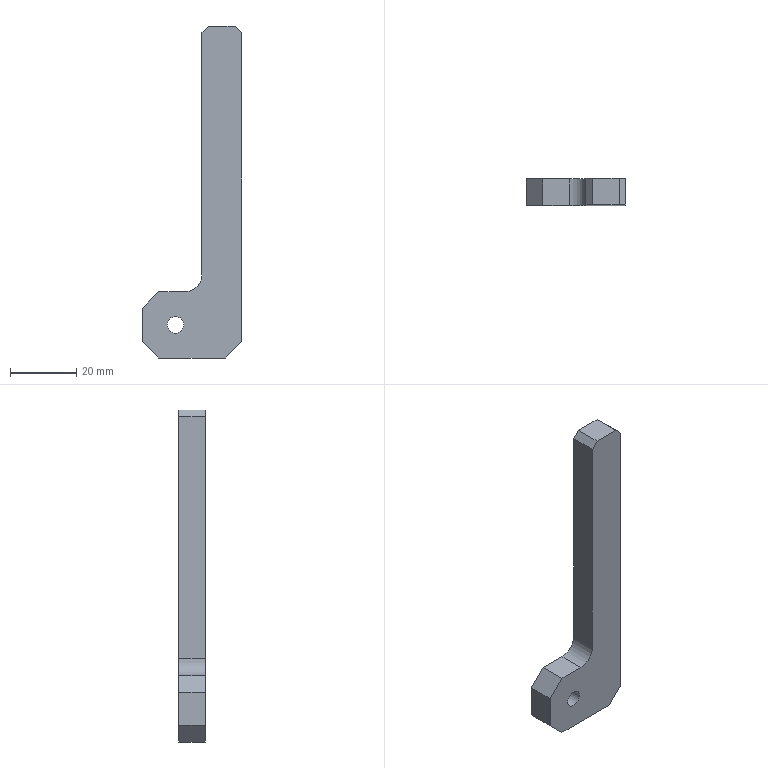Part | NX | features 5003_209_Plate 2 | 1 solid | 15 faces | box 30 x 8 x 100 mm | volume 12034 mm3 | plane 13 | cylinder 2 | commonest cylinder face diameters 5 x1 10 x1
STEP:
#1=CARTESIAN_POINT('',(-208.775,-608.606,-95.5));
#2=VERTEX_POINT('',#1);
#3=CARTESIAN_POINT('',(-208.775,-608.606,-22.5));
#4=VERTEX_POINT('',#3);
#5=CARTESIAN_POINT('',(-208.775,-608.606,-95.5));
#6=DIRECTION('',(0.,0.,1.));
#7=VECTOR('',#6,1000.);
#8=LINE('',#5,#7);
#9=EDGE_CURVE('',#2,#4,#8,.T.);
#10=ORIENTED_EDGE('',*,*,#9,.T.);
#11=CARTESIAN_POINT('',(-206.775,-608.606,-20.5));
#12=VERTEX_POINT('',#11);
#13=CARTESIAN_POINT('',(-247.775,-608.606,-61.5));
#14=DIRECTION('',(-0.7071,0.,-0.7071));
#15=VECTOR('',#14,1000.);
#16=LINE('',#13,#15);
#17=EDGE_CURVE('',#4,#12,#16,.F.);
#18=ORIENTED_EDGE('',*,*,#17,.T.);
#19=CARTESIAN_POINT('',(-198.775,-608.606,-20.5));
#20=VERTEX_POINT('',#19);
#21=CARTESIAN_POINT('',(-196.775,-608.606,-20.5));
#22=DIRECTION('',(1.,0.,0.));
#23=VECTOR('',#22,1000.);
#24=LINE('',#21,#23);
#25=EDGE_CURVE('',#12,#20,#24,.T.);
#26=ORIENTED_EDGE('',*,*,#25,.T.);
#27=CARTESIAN_POINT('',(-196.775,-608.606,-22.5));
#28=VERTEX_POINT('',#27);
#29=CARTESIAN_POINT('',(-168.775,-608.606,-50.5));
#30=DIRECTION('',(-0.7071,0.,0.7071));
#31=VECTOR('',#30,1000.);
#32=LINE('',#29,#31);
#33=EDGE_CURVE('',#20,#28,#32,.F.);
#34=ORIENTED_EDGE('',*,*,#33,.T.);
#35=CARTESIAN_POINT('',(-196.775,-608.606,-115.5));
#36=VERTEX_POINT('',#35);
#37=CARTESIAN_POINT('',(-196.775,-608.606,-115.5));
#38=DIRECTION('',(0.,0.,-1.));
#39=VECTOR('',#38,1000.);
#40=LINE('',#37,#39);
#41=EDGE_CURVE('',#28,#36,#40,.T.);
#42=ORIENTED_EDGE('',*,*,#41,.T.);
#43=CARTESIAN_POINT('',(-201.775,-608.606,-120.5));
#44=VERTEX_POINT('',#43);
#45=CARTESIAN_POINT('',(-201.775,-608.606,-120.5));
#46=DIRECTION('',(-0.7071,0.,-0.7071));
#47=VECTOR('',#46,1000.);
#48=LINE('',#45,#47);
#49=EDGE_CURVE('',#36,#44,#48,.T.);
#50=ORIENTED_EDGE('',*,*,#49,.T.);
#51=CARTESIAN_POINT('',(-221.775,-608.606,-120.5));
#52=VERTEX_POINT('',#51);
#53=CARTESIAN_POINT('',(-201.775,-608.606,-120.5));
#54=DIRECTION('',(-1.,0.,0.));
#55=VECTOR('',#54,1000.);
#56=LINE('',#53,#55);
#57=EDGE_CURVE('',#44,#52,#56,.T.);
#58=ORIENTED_EDGE('',*,*,#57,.T.);
#59=CARTESIAN_POINT('',(-226.775,-608.606,-115.5));
#60=VERTEX_POINT('',#59);
#61=CARTESIAN_POINT('',(-226.775,-608.606,-115.5));
#62=DIRECTION('',(-0.7071,0.,0.7071));
#63=VECTOR('',#62,1000.);
#64=LINE('',#61,#63);
#65=EDGE_CURVE('',#52,#60,#64,.T.);
#66=ORIENTED_EDGE('',*,*,#65,.T.);
#67=CARTESIAN_POINT('',(-226.775,-608.606,-105.5));
#68=VERTEX_POINT('',#67);
#69=CARTESIAN_POINT('',(-226.775,-608.606,-105.5));
#70=DIRECTION('',(0.,0.,1.));
#71=VECTOR('',#70,1000.);
#72=LINE('',#69,#71);
#73=EDGE_CURVE('',#60,#68,#72,.T.);
#74=ORIENTED_EDGE('',*,*,#73,.T.);
#75=CARTESIAN_POINT('',(-221.775,-608.606,-100.5));
#76=VERTEX_POINT('',#75);
#77=CARTESIAN_POINT('',(-221.775,-608.606,-100.5));
#78=DIRECTION('',(0.7071,0.,0.7071));
#79=VECTOR('',#78,1000.);
#80=LINE('',#77,#79);
#81=EDGE_CURVE('',#68,#76,#80,.T.);
#82=ORIENTED_EDGE('',*,*,#81,.T.);
#83=CARTESIAN_POINT('',(-213.775,-608.606,-100.5));
#84=VERTEX_POINT('',#83);
#85=CARTESIAN_POINT('',(-213.775,-608.606,-100.5));
#86=DIRECTION('',(1.,0.,0.));
#87=VECTOR('',#86,1000.);
#88=LINE('',#85,#87);
#89=EDGE_CURVE('',#76,#84,#88,.T.);
#90=ORIENTED_EDGE('',*,*,#89,.T.);
#91=CARTESIAN_POINT('',(-213.775,-608.606,-95.5));
#92=DIRECTION('',(0.,-1.,0.));
#93=DIRECTION('',(-1.,0.,0.));
#94=AXIS2_PLACEMENT_3D('',#91,#92,#93);
#95=CIRCLE('',#94,5.);
#96=EDGE_CURVE('',#84,#2,#95,.T.);
#97=ORIENTED_EDGE('',*,*,#96,.T.);
#98=EDGE_LOOP('',(#10,#18,#26,#34,#42,#50,#58,#66,#74,#82,#90,#97));
#99=FACE_BOUND('',#98,.T.);
#100=CARTESIAN_POINT('',(-219.275,-608.606,-110.5));
#101=VERTEX_POINT('',#100);
#102=CARTESIAN_POINT('',(-216.775,-608.606,-110.5));
#103=DIRECTION('',(0.,1.,0.));
#104=DIRECTION('',(-1.,0.,0.));
#105=AXIS2_PLACEMENT_3D('',#102,#103,#104);
#106=CIRCLE('',#105,2.5);
#107=EDGE_CURVE('',#101,#101,#106,.T.);
#108=ORIENTED_EDGE('',*,*,#107,.F.);
#109=EDGE_LOOP('',(#108));
#110=FACE_BOUND('',#109,.T.);
#111=CARTESIAN_POINT('',(-213.775,-608.606,-95.5));
#112=DIRECTION('',(0.,1.,0.));
#113=DIRECTION('',(-1.,0.,0.));
#114=AXIS2_PLACEMENT_3D('',#111,#112,#113);
#115=PLANE('',#114);
#116=ADVANCED_FACE('',(#99,#110),#115,.T.);
#117=CARTESIAN_POINT('',(-206.775,-616.606,-20.5));
#118=VERTEX_POINT('',#117);
#119=CARTESIAN_POINT('',(-198.775,-616.606,-20.5));
#120=VERTEX_POINT('',#119);
#121=CARTESIAN_POINT('',(-196.775,-616.606,-20.5));
#122=DIRECTION('',(1.,0.,0.));
#123=VECTOR('',#122,1000.);
#124=LINE('',#121,#123);
#125=EDGE_CURVE('',#118,#120,#124,.T.);
#126=ORIENTED_EDGE('',*,*,#125,.F.);
#127=CARTESIAN_POINT('',(-208.775,-616.606,-22.5));
#128=VERTEX_POINT('',#127);
#129=CARTESIAN_POINT('',(-206.775,-616.606,-20.5));
#130=DIRECTION('',(0.7071,0.,0.7071));
#131=VECTOR('',#130,1000.);
#132=LINE('',#129,#131);
#133=EDGE_CURVE('',#118,#128,#132,.F.);
#134=ORIENTED_EDGE('',*,*,#133,.T.);
#135=CARTESIAN_POINT('',(-208.775,-616.606,-95.5));
#136=VERTEX_POINT('',#135);
#137=CARTESIAN_POINT('',(-208.775,-616.606,-95.5));
#138=DIRECTION('',(0.,0.,1.));
#139=VECTOR('',#138,1000.);
#140=LINE('',#137,#139);
#141=EDGE_CURVE('',#136,#128,#140,.T.);
#142=ORIENTED_EDGE('',*,*,#141,.F.);
#143=CARTESIAN_POINT('',(-213.775,-616.606,-100.5));
#144=VERTEX_POINT('',#143);
#145=CARTESIAN_POINT('',(-213.775,-616.606,-95.5));
#146=DIRECTION('',(0.,-1.,0.));
#147=DIRECTION('',(-1.,0.,0.));
#148=AXIS2_PLACEMENT_3D('',#145,#146,#147);
#149=CIRCLE('',#148,5.);
#150=EDGE_CURVE('',#144,#136,#149,.T.);
#151=ORIENTED_EDGE('',*,*,#150,.F.);
#152=CARTESIAN_POINT('',(-221.775,-616.606,-100.5));
#153=VERTEX_POINT('',#152);
#154=CARTESIAN_POINT('',(-213.775,-616.606,-100.5));
#155=DIRECTION('',(1.,0.,0.));
#156=VECTOR('',#155,1000.);
#157=LINE('',#154,#156);
#158=EDGE_CURVE('',#153,#144,#157,.T.);
#159=ORIENTED_EDGE('',*,*,#158,.F.);
#160=CARTESIAN_POINT('',(-226.775,-616.606,-105.5));
#161=VERTEX_POINT('',#160);
#162=CARTESIAN_POINT('',(-221.775,-616.606,-100.5));
#163=DIRECTION('',(0.7071,0.,0.7071));
#164=VECTOR('',#163,1000.);
#165=LINE('',#162,#164);
#166=EDGE_CURVE('',#161,#153,#165,.T.);
#167=ORIENTED_EDGE('',*,*,#166,.F.);
#168=CARTESIAN_POINT('',(-226.775,-616.606,-115.5));
#169=VERTEX_POINT('',#168);
#170=CARTESIAN_POINT('',(-226.775,-616.606,-105.5));
#171=DIRECTION('',(0.,0.,1.));
#172=VECTOR('',#171,1000.);
#173=LINE('',#170,#172);
#174=EDGE_CURVE('',#169,#161,#173,.T.);
#175=ORIENTED_EDGE('',*,*,#174,.F.);
#176=CARTESIAN_POINT('',(-221.775,-616.606,-120.5));
#177=VERTEX_POINT('',#176);
#178=CARTESIAN_POINT('',(-226.775,-616.606,-115.5));
#179=DIRECTION('',(-0.7071,0.,0.7071));
#180=VECTOR('',#179,1000.);
#181=LINE('',#178,#180);
#182=EDGE_CURVE('',#177,#169,#181,.T.);
#183=ORIENTED_EDGE('',*,*,#182,.F.);
#184=CARTESIAN_POINT('',(-201.775,-616.606,-120.5));
#185=VERTEX_POINT('',#184);
#186=CARTESIAN_POINT('',(-201.775,-616.606,-120.5));
#187=DIRECTION('',(-1.,0.,0.));
#188=VECTOR('',#187,1000.);
#189=LINE('',#186,#188);
#190=EDGE_CURVE('',#185,#177,#189,.T.);
#191=ORIENTED_EDGE('',*,*,#190,.F.);
#192=CARTESIAN_POINT('',(-196.775,-616.606,-115.5));
#193=VERTEX_POINT('',#192);
#194=CARTESIAN_POINT('',(-201.775,-616.606,-120.5));
#195=DIRECTION('',(-0.7071,0.,-0.7071));
#196=VECTOR('',#195,1000.);
#197=LINE('',#194,#196);
#198=EDGE_CURVE('',#193,#185,#197,.T.);
#199=ORIENTED_EDGE('',*,*,#198,.F.);
#200=CARTESIAN_POINT('',(-196.775,-616.606,-22.5));
#201=VERTEX_POINT('',#200);
#202=CARTESIAN_POINT('',(-196.775,-616.606,-115.5));
#203=DIRECTION('',(0.,0.,-1.));
#204=VECTOR('',#203,1000.);
#205=LINE('',#202,#204);
#206=EDGE_CURVE('',#201,#193,#205,.T.);
#207=ORIENTED_EDGE('',*,*,#206,.F.);
#208=CARTESIAN_POINT('',(-196.775,-616.606,-22.5));
#209=DIRECTION('',(0.7071,0.,-0.7071));
#210=VECTOR('',#209,1000.);
#211=LINE('',#208,#210);
#212=EDGE_CURVE('',#201,#120,#211,.F.);
#213=ORIENTED_EDGE('',*,*,#212,.T.);
#214=EDGE_LOOP('',(#126,#134,#142,#151,#159,#167,#175,#183,#191,#199,#207,#213));
#215=FACE_BOUND('',#214,.T.);
#216=CARTESIAN_POINT('',(-219.275,-616.606,-110.5));
#217=VERTEX_POINT('',#216);
#218=CARTESIAN_POINT('',(-216.775,-616.606,-110.5));
#219=DIRECTION('',(0.,1.,0.));
#220=DIRECTION('',(-1.,0.,0.));
#221=AXIS2_PLACEMENT_3D('',#218,#219,#220);
#222=CIRCLE('',#221,2.5);
#223=EDGE_CURVE('',#217,#217,#222,.T.);
#224=ORIENTED_EDGE('',*,*,#223,.T.);
#225=EDGE_LOOP('',(#224));
#226=FACE_BOUND('',#225,.T.);
#227=CARTESIAN_POINT('',(-213.775,-616.606,-95.5));
#228=DIRECTION('',(0.,1.,0.));
#229=DIRECTION('',(-1.,0.,0.));
#230=AXIS2_PLACEMENT_3D('',#227,#228,#229);
#231=PLANE('',#230);
#232=ADVANCED_FACE('',(#215,#226),#231,.F.);
#233=ORIENTED_EDGE('',*,*,#141,.T.);
#234=CARTESIAN_POINT('',(-208.775,-608.606,-22.5));
#235=DIRECTION('',(0.,1.,0.));
#236=VECTOR('',#235,1000.);
#237=LINE('',#234,#236);
#238=EDGE_CURVE('',#128,#4,#237,.T.);
#239=ORIENTED_EDGE('',*,*,#238,.T.);
#240=ORIENTED_EDGE('',*,*,#9,.F.);
#241=CARTESIAN_POINT('',(-208.775,-608.606,-95.5));
#242=DIRECTION('',(0.,-1.,0.));
#243=VECTOR('',#242,1000.);
#244=LINE('',#241,#243);
#245=EDGE_CURVE('',#2,#136,#244,.T.);
#246=ORIENTED_EDGE('',*,*,#245,.T.);
#247=EDGE_LOOP('',(#233,#239,#240,#246));
#248=FACE_BOUND('',#247,.T.);
#249=CARTESIAN_POINT('',(-208.775,-608.606,-95.5));
#250=DIRECTION('',(1.,0.,0.));
#251=DIRECTION('',(0.,1.,0.));
#252=AXIS2_PLACEMENT_3D('',#249,#250,#251);
#253=PLANE('',#252);
#254=ADVANCED_FACE('',(#248),#253,.F.);
#255=ORIENTED_EDGE('',*,*,#25,.F.);
#256=CARTESIAN_POINT('',(-206.775,-608.606,-20.5));
#257=DIRECTION('',(0.,-1.,0.));
#258=VECTOR('',#257,1000.);
#259=LINE('',#256,#258);
#260=EDGE_CURVE('',#12,#118,#259,.T.);
#261=ORIENTED_EDGE('',*,*,#260,.T.);
#262=ORIENTED_EDGE('',*,*,#125,.T.);
#263=CARTESIAN_POINT('',(-198.775,-608.606,-20.5));
#264=DIRECTION('',(0.,1.,0.));
#265=VECTOR('',#264,1000.);
#266=LINE('',#263,#265);
#267=EDGE_CURVE('',#120,#20,#266,.T.);
#268=ORIENTED_EDGE('',*,*,#267,.T.);
#269=EDGE_LOOP('',(#255,#261,#262,#268));
#270=FACE_BOUND('',#269,.T.);
#271=CARTESIAN_POINT('',(-196.775,-608.606,-20.5));
#272=DIRECTION('',(0.,0.,-1.));
#273=DIRECTION('',(0.,-1.,0.));
#274=AXIS2_PLACEMENT_3D('',#271,#272,#273);
#275=PLANE('',#274);
#276=ADVANCED_FACE('',(#270),#275,.F.);
#277=ORIENTED_EDGE('',*,*,#41,.F.);
#278=CARTESIAN_POINT('',(-196.775,-608.606,-22.5));
#279=DIRECTION('',(0.,-1.,0.));
#280=VECTOR('',#279,1000.);
#281=LINE('',#278,#280);
#282=EDGE_CURVE('',#28,#201,#281,.T.);
#283=ORIENTED_EDGE('',*,*,#282,.T.);
#284=ORIENTED_EDGE('',*,*,#206,.T.);
#285=CARTESIAN_POINT('',(-196.775,-608.606,-115.5));
#286=DIRECTION('',(0.,-1.,0.));
#287=VECTOR('',#286,1000.);
#288=LINE('',#285,#287);
#289=EDGE_CURVE('',#36,#193,#288,.T.);
#290=ORIENTED_EDGE('',*,*,#289,.F.);
#291=EDGE_LOOP('',(#277,#283,#284,#290));
#292=FACE_BOUND('',#291,.T.);
#293=CARTESIAN_POINT('',(-196.775,-608.606,-115.5));
#294=DIRECTION('',(-1.,0.,0.));
#295=DIRECTION('',(0.,-1.,0.));
#296=AXIS2_PLACEMENT_3D('',#293,#294,#295);
#297=PLANE('',#296);
#298=ADVANCED_FACE('',(#292),#297,.F.);
#299=ORIENTED_EDGE('',*,*,#198,.T.);
#300=CARTESIAN_POINT('',(-201.775,-608.606,-120.5));
#301=DIRECTION('',(0.,-1.,0.));
#302=VECTOR('',#301,1000.);
#303=LINE('',#300,#302);
#304=EDGE_CURVE('',#44,#185,#303,.T.);
#305=ORIENTED_EDGE('',*,*,#304,.F.);
#306=ORIENTED_EDGE('',*,*,#49,.F.);
#307=ORIENTED_EDGE('',*,*,#289,.T.);
#308=EDGE_LOOP('',(#299,#305,#306,#307));
#309=FACE_BOUND('',#308,.T.);
#310=CARTESIAN_POINT('',(-201.775,-608.606,-120.5));
#311=DIRECTION('',(-0.7071,0.,0.7071));
#312=DIRECTION('',(0.7071,0.,0.7071));
#313=AXIS2_PLACEMENT_3D('',#310,#311,#312);
#314=PLANE('',#313);
#315=ADVANCED_FACE('',(#309),#314,.F.);
#316=ORIENTED_EDGE('',*,*,#190,.T.);
#317=CARTESIAN_POINT('',(-221.775,-608.606,-120.5));
#318=DIRECTION('',(0.,-1.,0.));
#319=VECTOR('',#318,1000.);
#320=LINE('',#317,#319);
#321=EDGE_CURVE('',#52,#177,#320,.T.);
#322=ORIENTED_EDGE('',*,*,#321,.F.);
#323=ORIENTED_EDGE('',*,*,#57,.F.);
#324=ORIENTED_EDGE('',*,*,#304,.T.);
#325=EDGE_LOOP('',(#316,#322,#323,#324));
#326=FACE_BOUND('',#325,.T.);
#327=CARTESIAN_POINT('',(-201.775,-608.606,-120.5));
#328=DIRECTION('',(0.,0.,1.));
#329=DIRECTION('',(0.,1.,0.));
#330=AXIS2_PLACEMENT_3D('',#327,#328,#329);
#331=PLANE('',#330);
#332=ADVANCED_FACE('',(#326),#331,.F.);
#333=ORIENTED_EDGE('',*,*,#182,.T.);
#334=CARTESIAN_POINT('',(-226.775,-608.606,-115.5));
#335=DIRECTION('',(0.,-1.,0.));
#336=VECTOR('',#335,1000.);
#337=LINE('',#334,#336);
#338=EDGE_CURVE('',#60,#169,#337,.T.);
#339=ORIENTED_EDGE('',*,*,#338,.F.);
#340=ORIENTED_EDGE('',*,*,#65,.F.);
#341=ORIENTED_EDGE('',*,*,#321,.T.);
#342=EDGE_LOOP('',(#333,#339,#340,#341));
#343=FACE_BOUND('',#342,.T.);
#344=CARTESIAN_POINT('',(-226.775,-608.606,-115.5));
#345=DIRECTION('',(0.7071,0.,0.7071));
#346=DIRECTION('',(0.7071,0.,-0.7071));
#347=AXIS2_PLACEMENT_3D('',#344,#345,#346);
#348=PLANE('',#347);
#349=ADVANCED_FACE('',(#343),#348,.F.);
#350=ORIENTED_EDGE('',*,*,#174,.T.);
#351=CARTESIAN_POINT('',(-226.775,-608.606,-105.5));
#352=DIRECTION('',(0.,-1.,0.));
#353=VECTOR('',#352,1000.);
#354=LINE('',#351,#353);
#355=EDGE_CURVE('',#68,#161,#354,.T.);
#356=ORIENTED_EDGE('',*,*,#355,.F.);
#357=ORIENTED_EDGE('',*,*,#73,.F.);
#358=ORIENTED_EDGE('',*,*,#338,.T.);
#359=EDGE_LOOP('',(#350,#356,#357,#358));
#360=FACE_BOUND('',#359,.T.);
#361=CARTESIAN_POINT('',(-226.775,-608.606,-105.5));
#362=DIRECTION('',(1.,0.,0.));
#363=DIRECTION('',(0.,0.,-1.));
#364=AXIS2_PLACEMENT_3D('',#361,#362,#363);
#365=PLANE('',#364);
#366=ADVANCED_FACE('',(#360),#365,.F.);
#367=ORIENTED_EDGE('',*,*,#166,.T.);
#368=CARTESIAN_POINT('',(-221.775,-608.606,-100.5));
#369=DIRECTION('',(0.,-1.,0.));
#370=VECTOR('',#369,1000.);
#371=LINE('',#368,#370);
#372=EDGE_CURVE('',#76,#153,#371,.T.);
#373=ORIENTED_EDGE('',*,*,#372,.F.);
#374=ORIENTED_EDGE('',*,*,#81,.F.);
#375=ORIENTED_EDGE('',*,*,#355,.T.);
#376=EDGE_LOOP('',(#367,#373,#374,#375));
#377=FACE_BOUND('',#376,.T.);
#378=CARTESIAN_POINT('',(-221.775,-608.606,-100.5));
#379=DIRECTION('',(0.7071,0.,-0.7071));
#380=DIRECTION('',(-0.7071,0.,-0.7071));
#381=AXIS2_PLACEMENT_3D('',#378,#379,#380);
#382=PLANE('',#381);
#383=ADVANCED_FACE('',(#377),#382,.F.);
#384=ORIENTED_EDGE('',*,*,#158,.T.);
#385=CARTESIAN_POINT('',(-213.775,-608.606,-100.5));
#386=DIRECTION('',(0.,-1.,0.));
#387=VECTOR('',#386,1000.);
#388=LINE('',#385,#387);
#389=EDGE_CURVE('',#84,#144,#388,.T.);
#390=ORIENTED_EDGE('',*,*,#389,.F.);
#391=ORIENTED_EDGE('',*,*,#89,.F.);
#392=ORIENTED_EDGE('',*,*,#372,.T.);
#393=EDGE_LOOP('',(#384,#390,#391,#392));
#394=FACE_BOUND('',#393,.T.);
#395=CARTESIAN_POINT('',(-213.775,-608.606,-100.5));
#396=DIRECTION('',(0.,0.,-1.));
#397=DIRECTION('',(0.,-1.,0.));
#398=AXIS2_PLACEMENT_3D('',#395,#396,#397);
#399=PLANE('',#398);
#400=ADVANCED_FACE('',(#394),#399,.F.);
#401=ORIENTED_EDGE('',*,*,#150,.T.);
#402=ORIENTED_EDGE('',*,*,#245,.F.);
#403=ORIENTED_EDGE('',*,*,#96,.F.);
#404=ORIENTED_EDGE('',*,*,#389,.T.);
#405=EDGE_LOOP('',(#401,#402,#403,#404));
#406=FACE_BOUND('',#405,.T.);
#407=CARTESIAN_POINT('',(-213.775,-608.606,-95.5));
#408=DIRECTION('',(0.,-1.,0.));
#409=DIRECTION('',(1.,0.,0.));
#410=AXIS2_PLACEMENT_3D('',#407,#408,#409);
#411=CYLINDRICAL_SURFACE('',#410,5.);
#412=ADVANCED_FACE('',(#406),#411,.F.);
#413=ORIENTED_EDGE('',*,*,#107,.T.);
#414=EDGE_LOOP('',(#413));
#415=FACE_BOUND('',#414,.T.);
#416=ORIENTED_EDGE('',*,*,#223,.F.);
#417=EDGE_LOOP('',(#416));
#418=FACE_BOUND('',#417,.T.);
#419=CARTESIAN_POINT('',(-216.775,-608.606,-110.5));
#420=DIRECTION('',(0.,-1.,0.));
#421=DIRECTION('',(1.,0.,0.));
#422=AXIS2_PLACEMENT_3D('',#419,#420,#421);
#423=CYLINDRICAL_SURFACE('',#422,2.5);
#424=ADVANCED_FACE('',(#415,#418),#423,.F.);
#425=ORIENTED_EDGE('',*,*,#17,.F.);
#426=ORIENTED_EDGE('',*,*,#238,.F.);
#427=ORIENTED_EDGE('',*,*,#133,.F.);
#428=ORIENTED_EDGE('',*,*,#260,.F.);
#429=EDGE_LOOP('',(#425,#426,#427,#428));
#430=FACE_BOUND('',#429,.T.);
#431=CARTESIAN_POINT('',(-206.775,-608.606,-20.5));
#432=DIRECTION('',(0.7071,0.,-0.7071));
#433=DIRECTION('',(0.,-1.,0.));
#434=AXIS2_PLACEMENT_3D('',#431,#432,#433);
#435=PLANE('',#434);
#436=ADVANCED_FACE('',(#430),#435,.F.);
#437=ORIENTED_EDGE('',*,*,#33,.F.);
#438=ORIENTED_EDGE('',*,*,#267,.F.);
#439=ORIENTED_EDGE('',*,*,#212,.F.);
#440=ORIENTED_EDGE('',*,*,#282,.F.);
#441=EDGE_LOOP('',(#437,#438,#439,#440));
#442=FACE_BOUND('',#441,.T.);
#443=CARTESIAN_POINT('',(-196.775,-608.606,-22.5));
#444=DIRECTION('',(-0.7071,0.,-0.7071));
#445=DIRECTION('',(0.,-1.,0.));
#446=AXIS2_PLACEMENT_3D('',#443,#444,#445);
#447=PLANE('',#446);
#448=ADVANCED_FACE('',(#442),#447,.F.);
#449=CLOSED_SHELL('',(#116,#232,#254,#276,#298,#315,#332,#349,#366,#383,#400,#412,#424,#436,#448));
#450=MANIFOLD_SOLID_BREP('',#449);
#451=(LENGTH_UNIT()NAMED_UNIT(*)SI_UNIT(.MILLI.,.METRE.));
#452=UNCERTAINTY_MEASURE_WITH_UNIT(LENGTH_MEASURE(0.00001),#451,'','');
#453=(NAMED_UNIT(*)PLANE_ANGLE_UNIT()SI_UNIT($,.RADIAN.));
#454=(NAMED_UNIT(*)SI_UNIT($,.STERADIAN.)SOLID_ANGLE_UNIT());
#455=(GEOMETRIC_REPRESENTATION_CONTEXT(3)GLOBAL_UNCERTAINTY_ASSIGNED_CONTEXT((#452))GLOBAL_UNIT_ASSIGNED_CONTEXT((#451,#453,#454))REPRESENTATION_CONTEXT('',''));
#456=ADVANCED_BREP_SHAPE_REPRESENTATION('',(#450),#455);